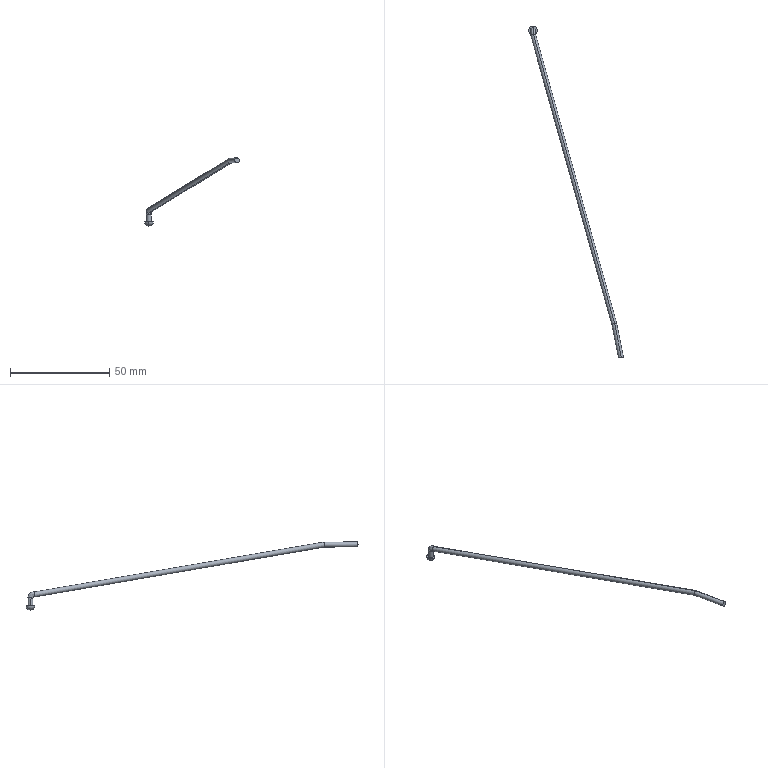Part | STEP file | Spoke_IN | 1 solid | 12 faces | box 47.785 x 167.549 x 34.429 mm | volume 896.22 mm3 | spline 6 | sphere 2 | cylinder 2 | plane 2 | commonest cylinder face diameters 2.5 x2